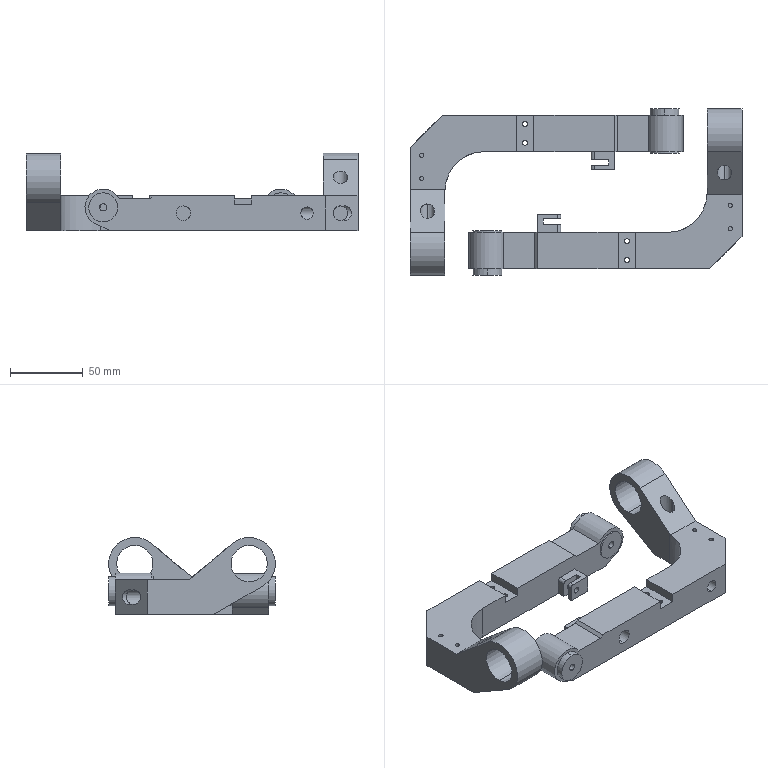Part | 2 solids | 150 faces | box 228 x 114.503 x 53 mm | volume 287677 mm3 | cylinder 84 | plane 66 | commonest cylinder face diameters 10 x22 3 x8 3.5 x8 4.1 x8 8.6 x8 20 x8